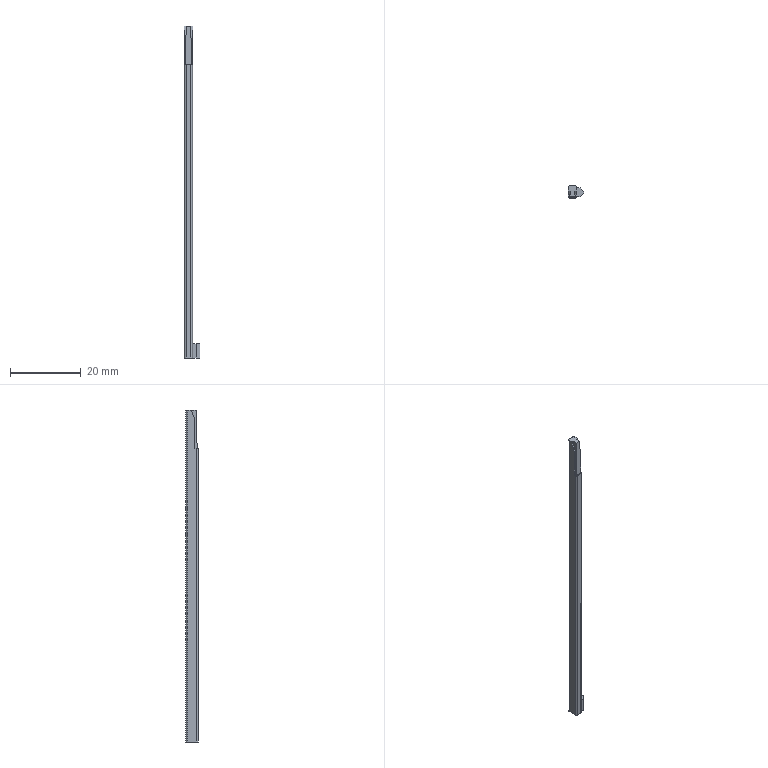Part | Creo | 1 solid | 24 faces | box 4.3 x 3.495 x 94.171 mm | volume 738.104 mm3 | plane 20 | cylinder 4 | commonest cylinder face diameters 1 x4
STEP:
#1=CARTESIAN_POINT('',(0.,0.,0.));
#2=DIRECTION('',(0.,0.,1.));
#3=DIRECTION('',(1.,0.,0.));
#4=AXIS2_PLACEMENT_3D('',#1,#2,#3);
#5=CARTESIAN_POINT('',(8.568,10.447,29.026));
#6=VERTEX_POINT('',#5);
#7=CARTESIAN_POINT('',(9.868,10.447,29.026));
#8=VERTEX_POINT('',#7);
#9=CARTESIAN_POINT('',(8.568,10.447,29.026));
#10=DIRECTION('',(1.,0.,0.));
#11=VECTOR('',#10,1.3);
#12=LINE('',#9,#11);
#13=EDGE_CURVE('',#6,#8,#12,.T.);
#14=ORIENTED_EDGE('',*,*,#13,.T.);
#15=CARTESIAN_POINT('',(9.868,10.447,-54.09));
#16=VERTEX_POINT('',#15);
#17=CARTESIAN_POINT('',(9.868,10.447,29.026));
#18=DIRECTION('',(0.,0.,-1.));
#19=VECTOR('',#18,83.116);
#20=LINE('',#17,#19);
#21=EDGE_CURVE('',#8,#16,#20,.T.);
#22=ORIENTED_EDGE('',*,*,#21,.T.);
#23=CARTESIAN_POINT('',(8.568,10.447,-54.09));
#24=VERTEX_POINT('',#23);
#25=CARTESIAN_POINT('',(9.868,10.447,-54.09));
#26=DIRECTION('',(-1.,0.,0.));
#27=VECTOR('',#26,1.3);
#28=LINE('',#25,#27);
#29=EDGE_CURVE('',#16,#24,#28,.T.);
#30=ORIENTED_EDGE('',*,*,#29,.T.);
#31=CARTESIAN_POINT('',(8.568,10.447,-54.09));
#32=DIRECTION('',(0.,0.,1.));
#33=VECTOR('',#32,83.116);
#34=LINE('',#31,#33);
#35=EDGE_CURVE('',#24,#6,#34,.T.);
#36=ORIENTED_EDGE('',*,*,#35,.T.);
#37=EDGE_LOOP('',(#14,#22,#30,#36));
#38=FACE_OUTER_BOUND('',#37,.F.);
#39=CARTESIAN_POINT('',(9.218,10.447,-59.974));
#40=DIRECTION('',(0.,-1.,0.));
#41=DIRECTION('',(0.,0.,-1.));
#42=AXIS2_PLACEMENT_3D('',#39,#40,#41);
#43=PLANE('',#42);
#44=ADVANCED_FACE('',(#38),#43,.T.);
#45=CARTESIAN_POINT('',(8.068,11.346,29.026));
#46=VERTEX_POINT('',#45);
#47=CARTESIAN_POINT('',(8.068,10.947,29.026));
#48=VERTEX_POINT('',#47);
#49=CARTESIAN_POINT('',(8.068,11.346,29.026));
#50=DIRECTION('',(0.,-1.,0.));
#51=VECTOR('',#50,0.399);
#52=LINE('',#49,#51);
#53=EDGE_CURVE('',#46,#48,#52,.T.);
#54=ORIENTED_EDGE('',*,*,#53,.F.);
#55=CARTESIAN_POINT('',(8.368,11.346,29.026));
#56=VERTEX_POINT('',#55);
#57=CARTESIAN_POINT('',(8.068,11.346,29.026));
#58=DIRECTION('',(1.,0.,0.));
#59=VECTOR('',#58,0.3);
#60=LINE('',#57,#59);
#61=EDGE_CURVE('',#46,#56,#60,.T.);
#62=ORIENTED_EDGE('',*,*,#61,.T.);
#63=CARTESIAN_POINT('',(8.368,10.747,29.026));
#64=VERTEX_POINT('',#63);
#65=CARTESIAN_POINT('',(8.368,11.346,29.026));
#66=DIRECTION('',(0.,-1.,0.));
#67=VECTOR('',#66,0.599);
#68=LINE('',#65,#67);
#69=EDGE_CURVE('',#56,#64,#68,.T.);
#70=ORIENTED_EDGE('',*,*,#69,.T.);
#71=CARTESIAN_POINT('',(10.068,10.747,29.026));
#72=VERTEX_POINT('',#71);
#73=CARTESIAN_POINT('',(8.368,10.747,29.026));
#74=DIRECTION('',(1.,0.,0.));
#75=VECTOR('',#74,1.7);
#76=LINE('',#73,#75);
#77=EDGE_CURVE('',#64,#72,#76,.T.);
#78=ORIENTED_EDGE('',*,*,#77,.T.);
#79=CARTESIAN_POINT('',(10.068,11.346,29.026));
#80=VERTEX_POINT('',#79);
#81=CARTESIAN_POINT('',(10.068,10.747,29.026));
#82=DIRECTION('',(0.,1.,0.));
#83=VECTOR('',#82,0.599);
#84=LINE('',#81,#83);
#85=EDGE_CURVE('',#72,#80,#84,.T.);
#86=ORIENTED_EDGE('',*,*,#85,.T.);
#87=CARTESIAN_POINT('',(10.368,11.346,29.026));
#88=VERTEX_POINT('',#87);
#89=CARTESIAN_POINT('',(10.068,11.346,29.026));
#90=DIRECTION('',(1.,0.,0.));
#91=VECTOR('',#90,0.3);
#92=LINE('',#89,#91);
#93=EDGE_CURVE('',#80,#88,#92,.T.);
#94=ORIENTED_EDGE('',*,*,#93,.T.);
#95=CARTESIAN_POINT('',(10.368,10.947,29.026));
#96=VERTEX_POINT('',#95);
#97=CARTESIAN_POINT('',(10.368,10.947,29.026));
#98=DIRECTION('',(0.,1.,0.));
#99=VECTOR('',#98,0.399);
#100=LINE('',#97,#99);
#101=EDGE_CURVE('',#96,#88,#100,.T.);
#102=ORIENTED_EDGE('',*,*,#101,.F.);
#103=CARTESIAN_POINT('',(9.868,10.947,29.026));
#104=DIRECTION('',(0.,0.,1.));
#105=DIRECTION('',(0.,-1.,0.));
#106=AXIS2_PLACEMENT_3D('',#103,#104,#105);
#107=CIRCLE('',#106,0.5);
#108=EDGE_CURVE('',#8,#96,#107,.T.);
#109=ORIENTED_EDGE('',*,*,#108,.F.);
#110=ORIENTED_EDGE('',*,*,#13,.F.);
#111=CARTESIAN_POINT('',(8.568,10.947,29.026));
#112=DIRECTION('',(0.,0.,1.));
#113=DIRECTION('',(-1.,0.,0.));
#114=AXIS2_PLACEMENT_3D('',#111,#112,#113);
#115=CIRCLE('',#114,0.5);
#116=EDGE_CURVE('',#48,#6,#115,.T.);
#117=ORIENTED_EDGE('',*,*,#116,.F.);
#118=EDGE_LOOP('',(#54,#62,#70,#78,#86,#94,#102,#109,#110,#117));
#119=FACE_OUTER_BOUND('',#118,.F.);
#120=CARTESIAN_POINT('',(-0.07825,-88.35,29.026));
#121=DIRECTION('',(0.,0.,-1.));
#122=DIRECTION('',(0.,-1.,0.));
#123=AXIS2_PLACEMENT_3D('',#120,#121,#122);
#124=PLANE('',#123);
#125=ADVANCED_FACE('',(#119),#124,.F.);
#126=CARTESIAN_POINT('',(8.068,11.418,37.282));
#127=VERTEX_POINT('',#126);
#128=CARTESIAN_POINT('',(8.068,12.351,40.081));
#129=VERTEX_POINT('',#128);
#130=CARTESIAN_POINT('',(8.068,11.418,37.282));
#131=DIRECTION('',(0.,0.3162,0.9487));
#132=VECTOR('',#131,2.95);
#133=LINE('',#130,#132);
#134=EDGE_CURVE('',#127,#129,#133,.T.);
#135=ORIENTED_EDGE('',*,*,#134,.F.);
#136=CARTESIAN_POINT('',(8.068,11.346,29.026));
#137=DIRECTION('',(0.,0.008727,1.));
#138=VECTOR('',#137,8.256);
#139=LINE('',#136,#138);
#140=EDGE_CURVE('',#46,#127,#139,.T.);
#141=ORIENTED_EDGE('',*,*,#140,.F.);
#142=ORIENTED_EDGE('',*,*,#53,.T.);
#143=CARTESIAN_POINT('',(8.068,10.947,-54.09));
#144=VERTEX_POINT('',#143);
#145=CARTESIAN_POINT('',(8.068,10.947,29.026));
#146=DIRECTION('',(0.,0.,-1.));
#147=VECTOR('',#146,83.116);
#148=LINE('',#145,#147);
#149=EDGE_CURVE('',#48,#144,#148,.T.);
#150=ORIENTED_EDGE('',*,*,#149,.T.);
#151=CARTESIAN_POINT('',(8.068,13.442,-54.09));
#152=VERTEX_POINT('',#151);
#153=CARTESIAN_POINT('',(8.068,10.947,-54.09));
#154=DIRECTION('',(0.,1.,0.));
#155=VECTOR('',#154,2.495);
#156=LINE('',#153,#155);
#157=EDGE_CURVE('',#144,#152,#156,.T.);
#158=ORIENTED_EDGE('',*,*,#157,.T.);
#159=CARTESIAN_POINT('',(8.068,13.442,40.081));
#160=VERTEX_POINT('',#159);
#161=CARTESIAN_POINT('',(8.068,13.442,-54.09));
#162=DIRECTION('',(0.,0.,1.));
#163=VECTOR('',#162,94.171);
#164=LINE('',#161,#163);
#165=EDGE_CURVE('',#152,#160,#164,.T.);
#166=ORIENTED_EDGE('',*,*,#165,.T.);
#167=CARTESIAN_POINT('',(8.068,12.351,40.081));
#168=DIRECTION('',(0.,1.,0.));
#169=VECTOR('',#168,1.091);
#170=LINE('',#167,#169);
#171=EDGE_CURVE('',#129,#160,#170,.T.);
#172=ORIENTED_EDGE('',*,*,#171,.F.);
#173=EDGE_LOOP('',(#135,#141,#142,#150,#158,#166,#172));
#174=FACE_OUTER_BOUND('',#173,.F.);
#175=CARTESIAN_POINT('',(8.068,11.945,-59.974));
#176=DIRECTION('',(-1.,0.,0.));
#177=DIRECTION('',(0.,0.,1.));
#178=AXIS2_PLACEMENT_3D('',#175,#176,#177);
#179=PLANE('',#178);
#180=ADVANCED_FACE('',(#174),#179,.T.);
#181=CARTESIAN_POINT('',(8.512,11.418,37.282));
#182=VERTEX_POINT('',#181);
#183=CARTESIAN_POINT('',(8.068,11.418,37.282));
#184=DIRECTION('',(1.,0.,0.));
#185=VECTOR('',#184,0.4441);
#186=LINE('',#183,#185);
#187=EDGE_CURVE('',#127,#182,#186,.T.);
#188=ORIENTED_EDGE('',*,*,#187,.F.);
#189=ORIENTED_EDGE('',*,*,#134,.T.);
#190=CARTESIAN_POINT('',(8.561,12.351,40.081));
#191=VERTEX_POINT('',#190);
#192=CARTESIAN_POINT('',(8.068,12.351,40.081));
#193=DIRECTION('',(1.,0.,0.));
#194=VECTOR('',#193,0.493);
#195=LINE('',#192,#194);
#196=EDGE_CURVE('',#129,#191,#195,.T.);
#197=ORIENTED_EDGE('',*,*,#196,.T.);
#198=CARTESIAN_POINT('',(8.512,11.418,37.282));
#199=DIRECTION('',(0.01656,0.3162,0.9486));
#200=VECTOR('',#199,2.951);
#201=LINE('',#198,#200);
#202=EDGE_CURVE('',#182,#191,#201,.T.);
#203=ORIENTED_EDGE('',*,*,#202,.F.);
#204=EDGE_LOOP('',(#188,#189,#197,#203));
#205=FACE_OUTER_BOUND('',#204,.F.);
#206=CARTESIAN_POINT('',(7.962,11.848,38.574));
#207=DIRECTION('',(0.,0.9487,-0.3162));
#208=DIRECTION('',(0.,-0.3162,-0.9487));
#209=AXIS2_PLACEMENT_3D('',#206,#207,#208);
#210=PLANE('',#209);
#211=ADVANCED_FACE('',(#205),#210,.F.);
#212=CARTESIAN_POINT('',(8.512,11.418,37.282));
#213=DIRECTION('',(-0.01745,-0.008725,-0.9998));
#214=VECTOR('',#213,8.258);
#215=LINE('',#212,#214);
#216=EDGE_CURVE('',#182,#56,#215,.T.);
#217=ORIENTED_EDGE('',*,*,#216,.T.);
#218=ORIENTED_EDGE('',*,*,#61,.F.);
#219=ORIENTED_EDGE('',*,*,#140,.T.);
#220=ORIENTED_EDGE('',*,*,#187,.T.);
#221=EDGE_LOOP('',(#217,#218,#219,#220));
#222=FACE_OUTER_BOUND('',#221,.F.);
#223=CARTESIAN_POINT('',(3.845,11.346,29.026));
#224=DIRECTION('',(0.,1.,-0.008727));
#225=DIRECTION('',(-1.,0.,0.));
#226=AXIS2_PLACEMENT_3D('',#223,#224,#225);
#227=PLANE('',#226);
#228=ADVANCED_FACE('',(#222),#227,.F.);
#229=ORIENTED_EDGE('',*,*,#202,.T.);
#230=CARTESIAN_POINT('',(8.561,10.94,40.081));
#231=VERTEX_POINT('',#230);
#232=CARTESIAN_POINT('',(8.561,12.351,40.081));
#233=DIRECTION('',(0.,-1.,0.));
#234=VECTOR('',#233,1.411);
#235=LINE('',#232,#234);
#236=EDGE_CURVE('',#191,#231,#235,.T.);
#237=ORIENTED_EDGE('',*,*,#236,.T.);
#238=CARTESIAN_POINT('',(8.561,10.94,40.081));
#239=DIRECTION('',(-0.01745,-0.01745,-0.9997));
#240=VECTOR('',#239,11.058);
#241=LINE('',#238,#240);
#242=EDGE_CURVE('',#231,#64,#241,.T.);
#243=ORIENTED_EDGE('',*,*,#242,.T.);
#244=ORIENTED_EDGE('',*,*,#69,.F.);
#245=ORIENTED_EDGE('',*,*,#216,.F.);
#246=EDGE_LOOP('',(#229,#237,#243,#244,#245));
#247=FACE_OUTER_BOUND('',#246,.F.);
#248=CARTESIAN_POINT('',(8.561,11.442,40.081));
#249=DIRECTION('',(0.9998,0.,-0.01745));
#250=DIRECTION('',(-0.01745,0.,-0.9998));
#251=AXIS2_PLACEMENT_3D('',#248,#249,#250);
#252=PLANE('',#251);
#253=ADVANCED_FACE('',(#247),#252,.F.);
#254=ORIENTED_EDGE('',*,*,#196,.F.);
#255=ORIENTED_EDGE('',*,*,#171,.T.);
#256=CARTESIAN_POINT('',(8.568,13.942,40.081));
#257=VERTEX_POINT('',#256);
#258=CARTESIAN_POINT('',(8.568,13.442,40.081));
#259=DIRECTION('',(0.,0.,1.));
#260=DIRECTION('',(0.,1.,0.));
#261=AXIS2_PLACEMENT_3D('',#258,#259,#260);
#262=CIRCLE('',#261,0.5);
#263=EDGE_CURVE('',#257,#160,#262,.T.);
#264=ORIENTED_EDGE('',*,*,#263,.F.);
#265=CARTESIAN_POINT('',(9.868,13.942,40.081));
#266=VERTEX_POINT('',#265);
#267=CARTESIAN_POINT('',(8.568,13.942,40.081));
#268=DIRECTION('',(1.,0.,0.));
#269=VECTOR('',#268,1.3);
#270=LINE('',#267,#269);
#271=EDGE_CURVE('',#257,#266,#270,.T.);
#272=ORIENTED_EDGE('',*,*,#271,.T.);
#273=CARTESIAN_POINT('',(10.368,13.442,40.081));
#274=VERTEX_POINT('',#273);
#275=CARTESIAN_POINT('',(9.868,13.442,40.081));
#276=DIRECTION('',(0.,0.,1.));
#277=DIRECTION('',(1.,0.,0.));
#278=AXIS2_PLACEMENT_3D('',#275,#276,#277);
#279=CIRCLE('',#278,0.5);
#280=EDGE_CURVE('',#274,#266,#279,.T.);
#281=ORIENTED_EDGE('',*,*,#280,.F.);
#282=CARTESIAN_POINT('',(10.368,12.351,40.081));
#283=VERTEX_POINT('',#282);
#284=CARTESIAN_POINT('',(10.368,13.442,40.081));
#285=DIRECTION('',(0.,-1.,0.));
#286=VECTOR('',#285,1.091);
#287=LINE('',#284,#286);
#288=EDGE_CURVE('',#274,#283,#287,.T.);
#289=ORIENTED_EDGE('',*,*,#288,.T.);
#290=CARTESIAN_POINT('',(9.875,12.351,40.081));
#291=VERTEX_POINT('',#290);
#292=CARTESIAN_POINT('',(9.875,12.351,40.081));
#293=DIRECTION('',(1.,0.,0.));
#294=VECTOR('',#293,0.493);
#295=LINE('',#292,#294);
#296=EDGE_CURVE('',#291,#283,#295,.T.);
#297=ORIENTED_EDGE('',*,*,#296,.F.);
#298=CARTESIAN_POINT('',(9.875,10.94,40.081));
#299=VERTEX_POINT('',#298);
#300=CARTESIAN_POINT('',(9.875,10.94,40.081));
#301=DIRECTION('',(0.,1.,0.));
#302=VECTOR('',#301,1.411);
#303=LINE('',#300,#302);
#304=EDGE_CURVE('',#299,#291,#303,.T.);
#305=ORIENTED_EDGE('',*,*,#304,.F.);
#306=CARTESIAN_POINT('',(8.561,10.94,40.081));
#307=DIRECTION('',(1.,0.,0.));
#308=VECTOR('',#307,1.315);
#309=LINE('',#306,#308);
#310=EDGE_CURVE('',#231,#299,#309,.T.);
#311=ORIENTED_EDGE('',*,*,#310,.F.);
#312=ORIENTED_EDGE('',*,*,#236,.F.);
#313=EDGE_LOOP('',(#254,#255,#264,#272,#281,#289,#297,#305,#311,#312));
#314=FACE_OUTER_BOUND('',#313,.F.);
#315=CARTESIAN_POINT('',(-17.817,-88.35,40.081));
#316=DIRECTION('',(0.,0.,1.));
#317=DIRECTION('',(-1.,0.,0.));
#318=AXIS2_PLACEMENT_3D('',#315,#316,#317);
#319=PLANE('',#318);
#320=ADVANCED_FACE('',(#314),#319,.T.);
#321=CARTESIAN_POINT('',(8.568,13.942,-54.09));
#322=VERTEX_POINT('',#321);
#323=CARTESIAN_POINT('',(8.568,13.442,-54.09));
#324=DIRECTION('',(0.,0.,-1.));
#325=DIRECTION('',(-1.,0.,0.));
#326=AXIS2_PLACEMENT_3D('',#323,#324,#325);
#327=CIRCLE('',#326,0.5);
#328=EDGE_CURVE('',#152,#322,#327,.T.);
#329=ORIENTED_EDGE('',*,*,#328,.T.);
#330=CARTESIAN_POINT('',(8.568,13.942,40.081));
#331=DIRECTION('',(0.,0.,-1.));
#332=VECTOR('',#331,94.171);
#333=LINE('',#330,#332);
#334=EDGE_CURVE('',#257,#322,#333,.T.);
#335=ORIENTED_EDGE('',*,*,#334,.F.);
#336=ORIENTED_EDGE('',*,*,#263,.T.);
#337=ORIENTED_EDGE('',*,*,#165,.F.);
#338=EDGE_LOOP('',(#329,#335,#336,#337));
#339=FACE_OUTER_BOUND('',#338,.F.);
#340=CARTESIAN_POINT('',(8.568,13.442,-59.974));
#341=DIRECTION('',(0.,0.,1.));
#342=DIRECTION('',(1.,0.,0.));
#343=AXIS2_PLACEMENT_3D('',#340,#341,#342);
#344=CYLINDRICAL_SURFACE('',#343,0.5);
#345=ADVANCED_FACE('',(#339),#344,.T.);
#346=CARTESIAN_POINT('',(10.368,13.442,-54.09));
#347=VERTEX_POINT('',#346);
#348=CARTESIAN_POINT('',(11.368,13.442,-54.09));
#349=VERTEX_POINT('',#348);
#350=CARTESIAN_POINT('',(10.368,13.442,-54.09));
#351=DIRECTION('',(1.,0.,0.));
#352=VECTOR('',#351,1.);
#353=LINE('',#350,#352);
#354=EDGE_CURVE('',#347,#349,#353,.T.);
#355=ORIENTED_EDGE('',*,*,#354,.F.);
#356=CARTESIAN_POINT('',(9.868,13.942,-54.09));
#357=VERTEX_POINT('',#356);
#358=CARTESIAN_POINT('',(9.868,13.442,-54.09));
#359=DIRECTION('',(0.,0.,-1.));
#360=DIRECTION('',(0.,1.,0.));
#361=AXIS2_PLACEMENT_3D('',#358,#359,#360);
#362=CIRCLE('',#361,0.5);
#363=EDGE_CURVE('',#357,#347,#362,.T.);
#364=ORIENTED_EDGE('',*,*,#363,.F.);
#365=CARTESIAN_POINT('',(8.568,13.942,-54.09));
#366=DIRECTION('',(1.,0.,0.));
#367=VECTOR('',#366,1.3);
#368=LINE('',#365,#367);
#369=EDGE_CURVE('',#322,#357,#368,.T.);
#370=ORIENTED_EDGE('',*,*,#369,.F.);
#371=ORIENTED_EDGE('',*,*,#328,.F.);
#372=ORIENTED_EDGE('',*,*,#157,.F.);
#373=CARTESIAN_POINT('',(8.568,10.947,-54.09));
#374=DIRECTION('',(0.,0.,-1.));
#375=DIRECTION('',(0.,-1.,0.));
#376=AXIS2_PLACEMENT_3D('',#373,#374,#375);
#377=CIRCLE('',#376,0.5);
#378=EDGE_CURVE('',#24,#144,#377,.T.);
#379=ORIENTED_EDGE('',*,*,#378,.F.);
#380=ORIENTED_EDGE('',*,*,#29,.F.);
#381=CARTESIAN_POINT('',(10.368,10.947,-54.09));
#382=VERTEX_POINT('',#381);
#383=CARTESIAN_POINT('',(9.868,10.947,-54.09));
#384=DIRECTION('',(0.,0.,-1.));
#385=DIRECTION('',(1.,0.,0.));
#386=AXIS2_PLACEMENT_3D('',#383,#384,#385);
#387=CIRCLE('',#386,0.5);
#388=EDGE_CURVE('',#382,#16,#387,.T.);
#389=ORIENTED_EDGE('',*,*,#388,.F.);
#390=CARTESIAN_POINT('',(11.368,10.947,-54.09));
#391=VERTEX_POINT('',#390);
#392=CARTESIAN_POINT('',(11.368,10.947,-54.09));
#393=DIRECTION('',(-1.,0.,0.));
#394=VECTOR('',#393,1.);
#395=LINE('',#392,#394);
#396=EDGE_CURVE('',#391,#382,#395,.T.);
#397=ORIENTED_EDGE('',*,*,#396,.F.);
#398=CARTESIAN_POINT('',(12.368,11.947,-54.09));
#399=VERTEX_POINT('',#398);
#400=CARTESIAN_POINT('',(12.368,11.947,-54.09));
#401=DIRECTION('',(-0.7071,-0.7071,0.));
#402=VECTOR('',#401,1.414);
#403=LINE('',#400,#402);
#404=EDGE_CURVE('',#399,#391,#403,.T.);
#405=ORIENTED_EDGE('',*,*,#404,.F.);
#406=CARTESIAN_POINT('',(12.368,12.442,-54.09));
#407=VERTEX_POINT('',#406);
#408=CARTESIAN_POINT('',(12.368,12.442,-54.09));
#409=DIRECTION('',(0.,-1.,0.));
#410=VECTOR('',#409,0.4955);
#411=LINE('',#408,#410);
#412=EDGE_CURVE('',#407,#399,#411,.T.);
#413=ORIENTED_EDGE('',*,*,#412,.F.);
#414=CARTESIAN_POINT('',(11.368,13.442,-54.09));
#415=DIRECTION('',(0.7071,-0.7071,0.));
#416=VECTOR('',#415,1.414);
#417=LINE('',#414,#416);
#418=EDGE_CURVE('',#349,#407,#417,.T.);
#419=ORIENTED_EDGE('',*,*,#418,.F.);
#420=EDGE_LOOP('',(#355,#364,#370,#371,#372,#379,#380,#389,#397,#405,#413,#419));
#421=FACE_OUTER_BOUND('',#420,.F.);
#422=CARTESIAN_POINT('',(0.,0.,-54.09));
#423=DIRECTION('',(0.,0.,-1.));
#424=DIRECTION('',(-1.,0.,0.));
#425=AXIS2_PLACEMENT_3D('',#422,#423,#424);
#426=PLANE('',#425);
#427=ADVANCED_FACE('',(#421),#426,.T.);
#428=CARTESIAN_POINT('',(11.368,13.442,-50.09));
#429=VERTEX_POINT('',#428);
#430=CARTESIAN_POINT('',(10.368,13.442,-50.09));
#431=VERTEX_POINT('',#430);
#432=CARTESIAN_POINT('',(11.368,13.442,-50.09));
#433=DIRECTION('',(-1.,0.,0.));
#434=VECTOR('',#433,1.);
#435=LINE('',#432,#434);
#436=EDGE_CURVE('',#429,#431,#435,.T.);
#437=ORIENTED_EDGE('',*,*,#436,.T.);
#438=CARTESIAN_POINT('',(10.368,13.442,-50.09));
#439=DIRECTION('',(0.,0.,-1.));
#440=VECTOR('',#439,4.);
#441=LINE('',#438,#440);
#442=EDGE_CURVE('',#431,#347,#441,.T.);
#443=ORIENTED_EDGE('',*,*,#442,.T.);
#444=ORIENTED_EDGE('',*,*,#354,.T.);
#445=CARTESIAN_POINT('',(11.368,13.442,-54.09));
#446=DIRECTION('',(0.,0.,1.));
#447=VECTOR('',#446,4.);
#448=LINE('',#445,#447);
#449=EDGE_CURVE('',#349,#429,#448,.T.);
#450=ORIENTED_EDGE('',*,*,#449,.T.);
#451=EDGE_LOOP('',(#437,#443,#444,#450));
#452=FACE_OUTER_BOUND('',#451,.F.);
#453=CARTESIAN_POINT('',(10.868,13.442,-54.09));
#454=DIRECTION('',(0.,1.,0.));
#455=DIRECTION('',(0.,0.,1.));
#456=AXIS2_PLACEMENT_3D('',#453,#454,#455);
#457=PLANE('',#456);
#458=ADVANCED_FACE('',(#452),#457,.T.);
#459=CARTESIAN_POINT('',(12.368,11.947,-50.09));
#460=VERTEX_POINT('',#459);
#461=CARTESIAN_POINT('',(12.368,12.442,-50.09));
#462=VERTEX_POINT('',#461);
#463=CARTESIAN_POINT('',(12.368,11.947,-50.09));
#464=DIRECTION('',(0.,1.,0.));
#465=VECTOR('',#464,0.4955);
#466=LINE('',#463,#465);
#467=EDGE_CURVE('',#460,#462,#466,.T.);
#468=ORIENTED_EDGE('',*,*,#467,.F.);
#469=CARTESIAN_POINT('',(11.368,10.947,-50.09));
#470=VERTEX_POINT('',#469);
#471=CARTESIAN_POINT('',(11.368,10.947,-50.09));
#472=DIRECTION('',(0.7071,0.7071,0.));
#473=VECTOR('',#472,1.414);
#474=LINE('',#471,#473);
#475=EDGE_CURVE('',#470,#460,#474,.T.);
#476=ORIENTED_EDGE('',*,*,#475,.F.);
#477=CARTESIAN_POINT('',(10.368,10.947,-50.09));
#478=VERTEX_POINT('',#477);
#479=CARTESIAN_POINT('',(10.368,10.947,-50.09));
#480=DIRECTION('',(1.,0.,0.));
#481=VECTOR('',#480,1.);
#482=LINE('',#479,#481);
#483=EDGE_CURVE('',#478,#470,#482,.T.);
#484=ORIENTED_EDGE('',*,*,#483,.F.);
#485=CARTESIAN_POINT('',(10.368,10.947,-50.09));
#486=DIRECTION('',(0.,1.,0.));
#487=VECTOR('',#486,2.495);
#488=LINE('',#485,#487);
#489=EDGE_CURVE('',#478,#431,#488,.T.);
#490=ORIENTED_EDGE('',*,*,#489,.T.);
#491=ORIENTED_EDGE('',*,*,#436,.F.);
#492=CARTESIAN_POINT('',(12.368,12.442,-50.09));
#493=DIRECTION('',(-0.7071,0.7071,0.));
#494=VECTOR('',#493,1.414);
#495=LINE('',#492,#494);
#496=EDGE_CURVE('',#462,#429,#495,.T.);
#497=ORIENTED_EDGE('',*,*,#496,.F.);
#498=EDGE_LOOP('',(#468,#476,#484,#490,#491,#497));
#499=FACE_OUTER_BOUND('',#498,.F.);
#500=CARTESIAN_POINT('',(10.868,12.195,-50.09));
#501=DIRECTION('',(0.,0.,1.));
#502=DIRECTION('',(1.,0.,0.));
#503=AXIS2_PLACEMENT_3D('',#500,#501,#502);
#504=PLANE('',#503);
#505=ADVANCED_FACE('',(#499),#504,.T.);
#506=ORIENTED_EDGE('',*,*,#412,.T.);
#507=CARTESIAN_POINT('',(12.368,11.947,-54.09));
#508=DIRECTION('',(0.,0.,1.));
#509=VECTOR('',#508,4.);
#510=LINE('',#507,#509);
#511=EDGE_CURVE('',#399,#460,#510,.T.);
#512=ORIENTED_EDGE('',*,*,#511,.T.);
#513=ORIENTED_EDGE('',*,*,#467,.T.);
#514=CARTESIAN_POINT('',(12.368,12.442,-50.09));
#515=DIRECTION('',(0.,0.,-1.));
#516=VECTOR('',#515,4.);
#517=LINE('',#514,#516);
#518=EDGE_CURVE('',#462,#407,#517,.T.);
#519=ORIENTED_EDGE('',*,*,#518,.T.);
#520=EDGE_LOOP('',(#506,#512,#513,#519));
#521=FACE_OUTER_BOUND('',#520,.F.);
#522=CARTESIAN_POINT('',(12.368,12.195,-54.09));
#523=DIRECTION('',(1.,0.,0.));
#524=DIRECTION('',(0.,0.,-1.));
#525=AXIS2_PLACEMENT_3D('',#522,#523,#524);
#526=PLANE('',#525);
#527=ADVANCED_FACE('',(#521),#526,.T.);
#528=ORIENTED_EDGE('',*,*,#404,.T.);
#529=CARTESIAN_POINT('',(11.368,10.947,-50.09));
#530=DIRECTION('',(0.,0.,-1.));
#531=VECTOR('',#530,4.);
#532=LINE('',#529,#531);
#533=EDGE_CURVE('',#470,#391,#532,.T.);
#534=ORIENTED_EDGE('',*,*,#533,.F.);
#535=ORIENTED_EDGE('',*,*,#475,.T.);
#536=ORIENTED_EDGE('',*,*,#511,.F.);
#537=EDGE_LOOP('',(#528,#534,#535,#536));
#538=FACE_OUTER_BOUND('',#537,.F.);
#539=CARTESIAN_POINT('',(11.368,10.947,-54.09));
#540=DIRECTION('',(-0.7071,0.7071,0.));
#541=DIRECTION('',(0.,0.,1.));
#542=AXIS2_PLACEMENT_3D('',#539,#540,#541);
#543=PLANE('',#542);
#544=ADVANCED_FACE('',(#538),#543,.F.);
#545=ORIENTED_EDGE('',*,*,#396,.T.);
#546=CARTESIAN_POINT('',(10.368,10.947,-54.09));
#547=DIRECTION('',(0.,0.,1.));
#548=VECTOR('',#547,4.);
#549=LINE('',#546,#548);
#550=EDGE_CURVE('',#382,#478,#549,.T.);
#551=ORIENTED_EDGE('',*,*,#550,.T.);
#552=ORIENTED_EDGE('',*,*,#483,.T.);
#553=ORIENTED_EDGE('',*,*,#533,.T.);
#554=EDGE_LOOP('',(#545,#551,#552,#553));
#555=FACE_OUTER_BOUND('',#554,.F.);
#556=CARTESIAN_POINT('',(10.868,10.947,-54.09));
#557=DIRECTION('',(0.,-1.,0.));
#558=DIRECTION('',(0.,0.,-1.));
#559=AXIS2_PLACEMENT_3D('',#556,#557,#558);
#560=PLANE('',#559);
#561=ADVANCED_FACE('',(#555),#560,.T.);
#562=ORIENTED_EDGE('',*,*,#388,.T.);
#563=ORIENTED_EDGE('',*,*,#21,.F.);
#564=ORIENTED_EDGE('',*,*,#108,.T.);
#565=CARTESIAN_POINT('',(10.368,10.947,-50.09));
#566=DIRECTION('',(0.,0.,1.));
#567=VECTOR('',#566,79.116);
#568=LINE('',#565,#567);
#569=EDGE_CURVE('',#478,#96,#568,.T.);
#570=ORIENTED_EDGE('',*,*,#569,.F.);
#571=ORIENTED_EDGE('',*,*,#550,.F.);
#572=EDGE_LOOP('',(#562,#563,#564,#570,#571));
#573=FACE_OUTER_BOUND('',#572,.F.);
#574=CARTESIAN_POINT('',(9.868,10.947,-59.974));
#575=DIRECTION('',(0.,0.,1.));
#576=DIRECTION('',(1.,0.,0.));
#577=AXIS2_PLACEMENT_3D('',#574,#575,#576);
#578=CYLINDRICAL_SURFACE('',#577,0.5);
#579=ADVANCED_FACE('',(#573),#578,.T.);
#580=CARTESIAN_POINT('',(10.368,11.418,37.282));
#581=VERTEX_POINT('',#580);
#582=CARTESIAN_POINT('',(10.368,12.351,40.081));
#583=DIRECTION('',(0.,-0.3162,-0.9487));
#584=VECTOR('',#583,2.95);
#585=LINE('',#582,#584);
#586=EDGE_CURVE('',#283,#581,#585,.T.);
#587=ORIENTED_EDGE('',*,*,#586,.F.);
#588=ORIENTED_EDGE('',*,*,#288,.F.);
#589=CARTESIAN_POINT('',(10.368,13.442,40.081));
#590=DIRECTION('',(0.,0.,-1.));
#591=VECTOR('',#590,90.171);
#592=LINE('',#589,#591);
#593=EDGE_CURVE('',#274,#431,#592,.T.);
#594=ORIENTED_EDGE('',*,*,#593,.T.);
#595=ORIENTED_EDGE('',*,*,#489,.F.);
#596=ORIENTED_EDGE('',*,*,#569,.T.);
#597=ORIENTED_EDGE('',*,*,#101,.T.);
#598=CARTESIAN_POINT('',(10.368,11.418,37.282));
#599=DIRECTION('',(0.,-0.008727,-1.));
#600=VECTOR('',#599,8.256);
#601=LINE('',#598,#600);
#602=EDGE_CURVE('',#581,#88,#601,.T.);
#603=ORIENTED_EDGE('',*,*,#602,.F.);
#604=EDGE_LOOP('',(#587,#588,#594,#595,#596,#597,#603));
#605=FACE_OUTER_BOUND('',#604,.F.);
#606=CARTESIAN_POINT('',(10.368,11.945,-59.974));
#607=DIRECTION('',(1.,0.,0.));
#608=DIRECTION('',(0.,0.,-1.));
#609=AXIS2_PLACEMENT_3D('',#606,#607,#608);
#610=PLANE('',#609);
#611=ADVANCED_FACE('',(#605),#610,.T.);
#612=CARTESIAN_POINT('',(9.924,11.418,37.282));
#613=VERTEX_POINT('',#612);
#614=CARTESIAN_POINT('',(9.924,11.418,37.282));
#615=DIRECTION('',(1.,0.,0.));
#616=VECTOR('',#615,0.4441);
#617=LINE('',#614,#616);
#618=EDGE_CURVE('',#613,#581,#617,.T.);
#619=ORIENTED_EDGE('',*,*,#618,.F.);
#620=CARTESIAN_POINT('',(9.875,12.351,40.081));
#621=DIRECTION('',(0.01656,-0.3162,-0.9486));
#622=VECTOR('',#621,2.951);
#623=LINE('',#620,#622);
#624=EDGE_CURVE('',#291,#613,#623,.T.);
#625=ORIENTED_EDGE('',*,*,#624,.F.);
#626=ORIENTED_EDGE('',*,*,#296,.T.);
#627=ORIENTED_EDGE('',*,*,#586,.T.);
#628=EDGE_LOOP('',(#619,#625,#626,#627));
#629=FACE_OUTER_BOUND('',#628,.F.);
#630=CARTESIAN_POINT('',(10.474,11.848,38.574));
#631=DIRECTION('',(0.,0.9487,-0.3162));
#632=DIRECTION('',(0.,-0.3162,-0.9487));
#633=AXIS2_PLACEMENT_3D('',#630,#631,#632);
#634=PLANE('',#633);
#635=ADVANCED_FACE('',(#629),#634,.F.);
#636=ORIENTED_EDGE('',*,*,#602,.T.);
#637=ORIENTED_EDGE('',*,*,#93,.F.);
#638=CARTESIAN_POINT('',(9.924,11.418,37.282));
#639=DIRECTION('',(0.01745,-0.008725,-0.9998));
#640=VECTOR('',#639,8.258);
#641=LINE('',#638,#640);
#642=EDGE_CURVE('',#613,#80,#641,.T.);
#643=ORIENTED_EDGE('',*,*,#642,.F.);
#644=ORIENTED_EDGE('',*,*,#618,.T.);
#645=EDGE_LOOP('',(#636,#637,#643,#644));
#646=FACE_OUTER_BOUND('',#645,.F.);
#647=CARTESIAN_POINT('',(6.357,11.346,29.026));
#648=DIRECTION('',(0.,1.,-0.008727));
#649=DIRECTION('',(-1.,0.,0.));
#650=AXIS2_PLACEMENT_3D('',#647,#648,#649);
#651=PLANE('',#650);
#652=ADVANCED_FACE('',(#646),#651,.F.);
#653=ORIENTED_EDGE('',*,*,#642,.T.);
#654=ORIENTED_EDGE('',*,*,#85,.F.);
#655=CARTESIAN_POINT('',(9.875,10.94,40.081));
#656=DIRECTION('',(0.01745,-0.01745,-0.9997));
#657=VECTOR('',#656,11.058);
#658=LINE('',#655,#657);
#659=EDGE_CURVE('',#299,#72,#658,.T.);
#660=ORIENTED_EDGE('',*,*,#659,.F.);
#661=ORIENTED_EDGE('',*,*,#304,.T.);
#662=ORIENTED_EDGE('',*,*,#624,.T.);
#663=EDGE_LOOP('',(#653,#654,#660,#661,#662));
#664=FACE_OUTER_BOUND('',#663,.F.);
#665=CARTESIAN_POINT('',(9.875,10.94,40.081));
#666=DIRECTION('',(-0.9998,0.,-0.01745));
#667=DIRECTION('',(-0.01745,0.,0.9998));
#668=AXIS2_PLACEMENT_3D('',#665,#666,#667);
#669=PLANE('',#668);
#670=ADVANCED_FACE('',(#664),#669,.F.);
#671=ORIENTED_EDGE('',*,*,#310,.T.);
#672=ORIENTED_EDGE('',*,*,#659,.T.);
#673=ORIENTED_EDGE('',*,*,#77,.F.);
#674=ORIENTED_EDGE('',*,*,#242,.F.);
#675=EDGE_LOOP('',(#671,#672,#673,#674));
#676=FACE_OUTER_BOUND('',#675,.F.);
#677=CARTESIAN_POINT('',(8.561,10.94,40.081));
#678=DIRECTION('',(0.,0.9998,-0.01745));
#679=DIRECTION('',(0.,-0.01745,-0.9998));
#680=AXIS2_PLACEMENT_3D('',#677,#678,#679);
#681=PLANE('',#680);
#682=ADVANCED_FACE('',(#676),#681,.F.);
#683=ORIENTED_EDGE('',*,*,#363,.T.);
#684=ORIENTED_EDGE('',*,*,#442,.F.);
#685=ORIENTED_EDGE('',*,*,#593,.F.);
#686=ORIENTED_EDGE('',*,*,#280,.T.);
#687=CARTESIAN_POINT('',(9.868,13.942,-54.09));
#688=DIRECTION('',(0.,0.,1.));
#689=VECTOR('',#688,94.171);
#690=LINE('',#687,#689);
#691=EDGE_CURVE('',#357,#266,#690,.T.);
#692=ORIENTED_EDGE('',*,*,#691,.F.);
#693=EDGE_LOOP('',(#683,#684,#685,#686,#692));
#694=FACE_OUTER_BOUND('',#693,.F.);
#695=CARTESIAN_POINT('',(9.868,13.442,-59.974));
#696=DIRECTION('',(0.,0.,1.));
#697=DIRECTION('',(1.,0.,0.));
#698=AXIS2_PLACEMENT_3D('',#695,#696,#697);
#699=CYLINDRICAL_SURFACE('',#698,0.5);
#700=ADVANCED_FACE('',(#694),#699,.T.);
#701=ORIENTED_EDGE('',*,*,#369,.T.);
#702=ORIENTED_EDGE('',*,*,#691,.T.);
#703=ORIENTED_EDGE('',*,*,#271,.F.);
#704=ORIENTED_EDGE('',*,*,#334,.T.);
#705=EDGE_LOOP('',(#701,#702,#703,#704));
#706=FACE_OUTER_BOUND('',#705,.F.);
#707=CARTESIAN_POINT('',(9.218,13.942,-59.974));
#708=DIRECTION('',(0.,1.,0.));
#709=DIRECTION('',(0.,0.,1.));
#710=AXIS2_PLACEMENT_3D('',#707,#708,#709);
#711=PLANE('',#710);
#712=ADVANCED_FACE('',(#706),#711,.T.);
#713=ORIENTED_EDGE('',*,*,#418,.T.);
#714=ORIENTED_EDGE('',*,*,#518,.F.);
#715=ORIENTED_EDGE('',*,*,#496,.T.);
#716=ORIENTED_EDGE('',*,*,#449,.F.);
#717=EDGE_LOOP('',(#713,#714,#715,#716));
#718=FACE_OUTER_BOUND('',#717,.F.);
#719=CARTESIAN_POINT('',(12.368,12.442,-54.09));
#720=DIRECTION('',(-0.7071,-0.7071,0.));
#721=DIRECTION('',(0.,0.,1.));
#722=AXIS2_PLACEMENT_3D('',#719,#720,#721);
#723=PLANE('',#722);
#724=ADVANCED_FACE('',(#718),#723,.F.);
#725=ORIENTED_EDGE('',*,*,#378,.T.);
#726=ORIENTED_EDGE('',*,*,#149,.F.);
#727=ORIENTED_EDGE('',*,*,#116,.T.);
#728=ORIENTED_EDGE('',*,*,#35,.F.);
#729=EDGE_LOOP('',(#725,#726,#727,#728));
#730=FACE_OUTER_BOUND('',#729,.F.);
#731=CARTESIAN_POINT('',(8.568,10.947,-59.974));
#732=DIRECTION('',(0.,0.,1.));
#733=DIRECTION('',(1.,0.,0.));
#734=AXIS2_PLACEMENT_3D('',#731,#732,#733);
#735=CYLINDRICAL_SURFACE('',#734,0.5);
#736=ADVANCED_FACE('',(#730),#735,.T.);
#737=CLOSED_SHELL('',(#44,#125,#180,#211,#228,#253,#320,#345,#427,#458,#505,#527,#544,#561,#579,#611,#635,#652,#670,#682,#700,#712,#724,#736));
#738=MANIFOLD_SOLID_BREP('',#737);
#739=(LENGTH_UNIT()NAMED_UNIT(*)SI_UNIT(.MILLI.,.METRE.));
#740=UNCERTAINTY_MEASURE_WITH_UNIT(LENGTH_MEASURE(0.009433),#739,'','');
#741=(NAMED_UNIT(*)PLANE_ANGLE_UNIT()SI_UNIT($,.RADIAN.));
#742=PLANE_ANGLE_MEASURE_WITH_UNIT(PLANE_ANGLE_MEASURE(0.01745),#741);
#743=(CONVERSION_BASED_UNIT('DEGREE',#742)NAMED_UNIT(*)PLANE_ANGLE_UNIT());
#744=(NAMED_UNIT(*)SI_UNIT($,.STERADIAN.)SOLID_ANGLE_UNIT());
#745=(GEOMETRIC_REPRESENTATION_CONTEXT(3)GLOBAL_UNCERTAINTY_ASSIGNED_CONTEXT((#740))GLOBAL_UNIT_ASSIGNED_CONTEXT((#739,#743,#744))REPRESENTATION_CONTEXT('',''));
#746=ADVANCED_BREP_SHAPE_REPRESENTATION('',(#4,#738),#745);